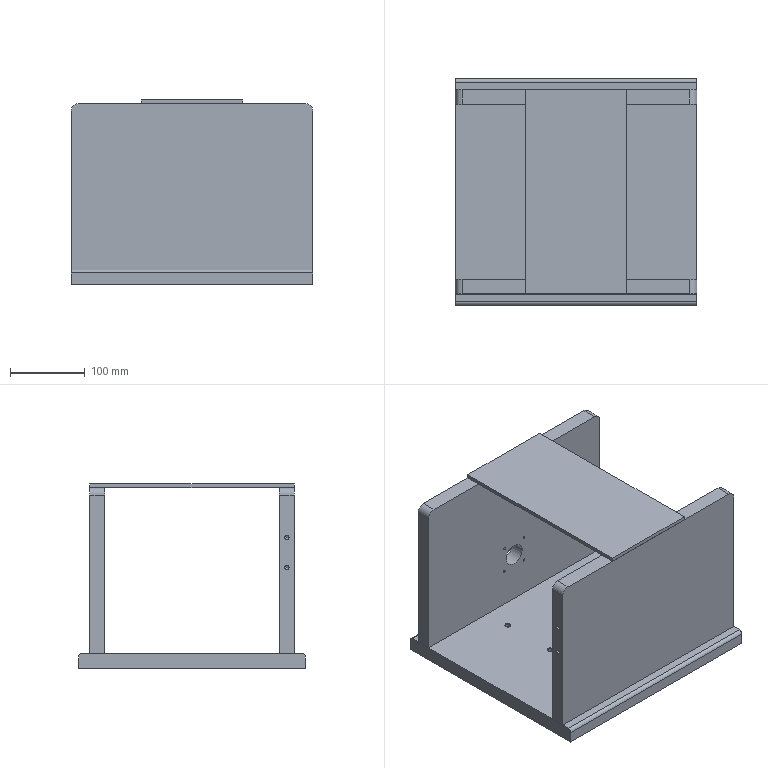Part | NX | features DATUM_CSYS 14, SKETCH 13, EXTRACT_FACE 10, HOLE PACKAGE 8, SIMPLE HOLE 8, SYMBOLIC_THREAD 8, Instance Feature 6, EXTRACT_STRING 5, EXTRUDE 5, Pattern Feature 3, BLEND 2, CHAMFER 1, Mirror Feature 1, Pattern Geometry 1 | 4 solids | 60 faces | box 324 x 304 x 247 mm | volume 5008657 mm3 | plane 24 | cylinder 19 | cone 17 | commonest cylinder face diameters 3.5 x4 5 x4 6.8 x4 20 x4 10 x2 30 x1
STEP:
#1=CARTESIAN_POINT('',(162.,289.,108.5));
#2=VERTEX_POINT('',#1);
#3=CARTESIAN_POINT('',(162.,289.,92.5));
#4=DIRECTION('',(0.,1.,0.));
#5=DIRECTION('',(0.,0.,1.));
#6=AXIS2_PLACEMENT_3D('',#3,#4,#5);
#7=CIRCLE('',#6,16.);
#8=EDGE_CURVE('',#2,#2,#7,.F.);
#9=ORIENTED_EDGE('',*,*,#8,.T.);
#10=EDGE_LOOP('',(#9));
#11=FACE_BOUND('',#10,.T.);
#12=CARTESIAN_POINT('',(143.438,289.,112.812));
#13=VERTEX_POINT('',#12);
#14=CARTESIAN_POINT('',(143.438,289.,111.062));
#15=DIRECTION('',(0.,1.,0.));
#16=DIRECTION('',(0.,0.,1.));
#17=AXIS2_PLACEMENT_3D('',#14,#15,#16);
#18=CIRCLE('',#17,1.75);
#19=EDGE_CURVE('',#13,#13,#18,.F.);
#20=ORIENTED_EDGE('',*,*,#19,.T.);
#21=EDGE_LOOP('',(#20));
#22=FACE_BOUND('',#21,.T.);
#23=CARTESIAN_POINT('',(143.438,289.,75.688));
#24=VERTEX_POINT('',#23);
#25=CARTESIAN_POINT('',(143.438,289.,73.938));
#26=DIRECTION('',(0.,1.,0.));
#27=DIRECTION('',(0.,0.,1.));
#28=AXIS2_PLACEMENT_3D('',#25,#26,#27);
#29=CIRCLE('',#28,1.75);
#30=EDGE_CURVE('',#24,#24,#29,.F.);
#31=ORIENTED_EDGE('',*,*,#30,.T.);
#32=EDGE_LOOP('',(#31));
#33=FACE_BOUND('',#32,.T.);
#34=CARTESIAN_POINT('',(180.562,289.,75.688));
#35=VERTEX_POINT('',#34);
#36=CARTESIAN_POINT('',(180.562,289.,73.938));
#37=DIRECTION('',(0.,1.,0.));
#38=DIRECTION('',(0.,0.,1.));
#39=AXIS2_PLACEMENT_3D('',#36,#37,#38);
#40=CIRCLE('',#39,1.75);
#41=EDGE_CURVE('',#35,#35,#40,.F.);
#42=ORIENTED_EDGE('',*,*,#41,.T.);
#43=EDGE_LOOP('',(#42));
#44=FACE_BOUND('',#43,.T.);
#45=CARTESIAN_POINT('',(180.562,289.,112.812));
#46=VERTEX_POINT('',#45);
#47=CARTESIAN_POINT('',(180.562,289.,111.062));
#48=DIRECTION('',(0.,1.,0.));
#49=DIRECTION('',(0.,0.,1.));
#50=AXIS2_PLACEMENT_3D('',#47,#48,#49);
#51=CIRCLE('',#50,1.75);
#52=EDGE_CURVE('',#46,#46,#51,.F.);
#53=ORIENTED_EDGE('',*,*,#52,.T.);
#54=EDGE_LOOP('',(#53));
#55=FACE_BOUND('',#54,.T.);
#56=CARTESIAN_POINT('',(0.,289.,232.));
#57=VERTEX_POINT('',#56);
#58=CARTESIAN_POINT('',(0.,289.,20.));
#59=VERTEX_POINT('',#58);
#60=CARTESIAN_POINT('',(0.,289.,242.));
#61=DIRECTION('',(0.,0.,-1.));
#62=VECTOR('',#61,1000.);
#63=LINE('',#60,#62);
#64=EDGE_CURVE('',#57,#59,#63,.T.);
#65=ORIENTED_EDGE('',*,*,#64,.F.);
#66=CARTESIAN_POINT('',(10.,289.,242.));
#67=VERTEX_POINT('',#66);
#68=CARTESIAN_POINT('',(10.,289.,232.));
#69=DIRECTION('',(0.,1.,0.));
#70=DIRECTION('',(0.,0.,1.));
#71=AXIS2_PLACEMENT_3D('',#68,#69,#70);
#72=CIRCLE('',#71,10.);
#73=EDGE_CURVE('',#57,#67,#72,.T.);
#74=ORIENTED_EDGE('',*,*,#73,.T.);
#75=CARTESIAN_POINT('',(314.,289.,242.));
#76=VERTEX_POINT('',#75);
#77=CARTESIAN_POINT('',(324.,289.,242.));
#78=DIRECTION('',(-1.,0.,0.));
#79=VECTOR('',#78,1000.);
#80=LINE('',#77,#79);
#81=EDGE_CURVE('',#76,#67,#80,.T.);
#82=ORIENTED_EDGE('',*,*,#81,.F.);
#83=CARTESIAN_POINT('',(324.,289.,232.));
#84=VERTEX_POINT('',#83);
#85=CARTESIAN_POINT('',(314.,289.,232.));
#86=DIRECTION('',(0.,1.,0.));
#87=DIRECTION('',(0.,0.,1.));
#88=AXIS2_PLACEMENT_3D('',#85,#86,#87);
#89=CIRCLE('',#88,10.);
#90=EDGE_CURVE('',#76,#84,#89,.T.);
#91=ORIENTED_EDGE('',*,*,#90,.T.);
#92=CARTESIAN_POINT('',(324.,289.,20.));
#93=VERTEX_POINT('',#92);
#94=CARTESIAN_POINT('',(324.,289.,242.));
#95=DIRECTION('',(0.,0.,-1.));
#96=VECTOR('',#95,1000.);
#97=LINE('',#94,#96);
#98=EDGE_CURVE('',#84,#93,#97,.T.);
#99=ORIENTED_EDGE('',*,*,#98,.T.);
#100=CARTESIAN_POINT('',(324.,289.,20.));
#101=DIRECTION('',(-1.,0.,0.));
#102=VECTOR('',#101,1000.);
#103=LINE('',#100,#102);
#104=EDGE_CURVE('',#93,#59,#103,.T.);
#105=ORIENTED_EDGE('',*,*,#104,.T.);
#106=EDGE_LOOP('',(#65,#74,#82,#91,#99,#105));
#107=FACE_BOUND('',#106,.T.);
#108=CARTESIAN_POINT('',(324.,289.,242.));
#109=DIRECTION('',(0.,1.,0.));
#110=DIRECTION('',(0.,0.,1.));
#111=AXIS2_PLACEMENT_3D('',#108,#109,#110);
#112=PLANE('',#111);
#113=ADVANCED_FACE('',(#11,#22,#33,#44,#55,#107),#112,.T.);
#114=CARTESIAN_POINT('',(0.,269.,20.));
#115=VERTEX_POINT('',#114);
#116=CARTESIAN_POINT('',(0.,289.,20.));
#117=DIRECTION('',(0.,-1.,0.));
#118=VECTOR('',#117,1000.);
#119=LINE('',#116,#118);
#120=EDGE_CURVE('',#59,#115,#119,.T.);
#121=ORIENTED_EDGE('',*,*,#120,.F.);
#122=ORIENTED_EDGE('',*,*,#104,.F.);
#123=CARTESIAN_POINT('',(324.,269.,20.));
#124=VERTEX_POINT('',#123);
#125=CARTESIAN_POINT('',(324.,289.,20.));
#126=DIRECTION('',(0.,-1.,0.));
#127=VECTOR('',#126,1000.);
#128=LINE('',#125,#127);
#129=EDGE_CURVE('',#93,#124,#128,.T.);
#130=ORIENTED_EDGE('',*,*,#129,.T.);
#131=CARTESIAN_POINT('',(324.,269.,20.));
#132=DIRECTION('',(-1.,0.,0.));
#133=VECTOR('',#132,1000.);
#134=LINE('',#131,#133);
#135=EDGE_CURVE('',#124,#115,#134,.T.);
#136=ORIENTED_EDGE('',*,*,#135,.T.);
#137=EDGE_LOOP('',(#121,#122,#130,#136));
#138=FACE_BOUND('',#137,.T.);
#139=CARTESIAN_POINT('',(324.,289.,20.));
#140=DIRECTION('',(0.,0.,-1.));
#141=DIRECTION('',(0.,1.,0.));
#142=AXIS2_PLACEMENT_3D('',#139,#140,#141);
#143=PLANE('',#142);
#144=ADVANCED_FACE('',(#138),#143,.T.);
#145=CARTESIAN_POINT('',(162.,269.,77.5));
#146=VERTEX_POINT('',#145);
#147=CARTESIAN_POINT('',(162.,269.,92.5));
#148=DIRECTION('',(0.,-1.,0.));
#149=DIRECTION('',(0.,0.,-1.));
#150=AXIS2_PLACEMENT_3D('',#147,#148,#149);
#151=CIRCLE('',#150,15.);
#152=EDGE_CURVE('',#146,#146,#151,.T.);
#153=ORIENTED_EDGE('',*,*,#152,.F.);
#154=EDGE_LOOP('',(#153));
#155=FACE_BOUND('',#154,.T.);
#156=CARTESIAN_POINT('',(143.438,269.,109.312));
#157=VERTEX_POINT('',#156);
#158=CARTESIAN_POINT('',(143.438,269.,111.062));
#159=DIRECTION('',(0.,-1.,0.));
#160=DIRECTION('',(0.,0.,-1.));
#161=AXIS2_PLACEMENT_3D('',#158,#159,#160);
#162=CIRCLE('',#161,1.75);
#163=EDGE_CURVE('',#157,#157,#162,.F.);
#164=ORIENTED_EDGE('',*,*,#163,.T.);
#165=EDGE_LOOP('',(#164));
#166=FACE_BOUND('',#165,.T.);
#167=CARTESIAN_POINT('',(143.438,269.,72.188));
#168=VERTEX_POINT('',#167);
#169=CARTESIAN_POINT('',(143.438,269.,73.938));
#170=DIRECTION('',(0.,-1.,0.));
#171=DIRECTION('',(0.,0.,-1.));
#172=AXIS2_PLACEMENT_3D('',#169,#170,#171);
#173=CIRCLE('',#172,1.75);
#174=EDGE_CURVE('',#168,#168,#173,.F.);
#175=ORIENTED_EDGE('',*,*,#174,.T.);
#176=EDGE_LOOP('',(#175));
#177=FACE_BOUND('',#176,.T.);
#178=CARTESIAN_POINT('',(180.562,269.,72.188));
#179=VERTEX_POINT('',#178);
#180=CARTESIAN_POINT('',(180.562,269.,73.938));
#181=DIRECTION('',(0.,-1.,0.));
#182=DIRECTION('',(0.,0.,-1.));
#183=AXIS2_PLACEMENT_3D('',#180,#181,#182);
#184=CIRCLE('',#183,1.75);
#185=EDGE_CURVE('',#179,#179,#184,.F.);
#186=ORIENTED_EDGE('',*,*,#185,.T.);
#187=EDGE_LOOP('',(#186));
#188=FACE_BOUND('',#187,.T.);
#189=CARTESIAN_POINT('',(180.562,269.,109.312));
#190=VERTEX_POINT('',#189);
#191=CARTESIAN_POINT('',(180.562,269.,111.062));
#192=DIRECTION('',(0.,-1.,0.));
#193=DIRECTION('',(0.,0.,-1.));
#194=AXIS2_PLACEMENT_3D('',#191,#192,#193);
#195=CIRCLE('',#194,1.75);
#196=EDGE_CURVE('',#190,#190,#195,.F.);
#197=ORIENTED_EDGE('',*,*,#196,.T.);
#198=EDGE_LOOP('',(#197));
#199=FACE_BOUND('',#198,.T.);
#200=CARTESIAN_POINT('',(314.,269.,242.));
#201=VERTEX_POINT('',#200);
#202=CARTESIAN_POINT('',(10.,269.,242.));
#203=VERTEX_POINT('',#202);
#204=CARTESIAN_POINT('',(324.,269.,242.));
#205=DIRECTION('',(-1.,0.,0.));
#206=VECTOR('',#205,1000.);
#207=LINE('',#204,#206);
#208=EDGE_CURVE('',#201,#203,#207,.T.);
#209=ORIENTED_EDGE('',*,*,#208,.T.);
#210=CARTESIAN_POINT('',(0.,269.,232.));
#211=VERTEX_POINT('',#210);
#212=CARTESIAN_POINT('',(10.,269.,232.));
#213=DIRECTION('',(0.,-1.,0.));
#214=DIRECTION('',(0.,0.,-1.));
#215=AXIS2_PLACEMENT_3D('',#212,#213,#214);
#216=CIRCLE('',#215,10.);
#217=EDGE_CURVE('',#203,#211,#216,.T.);
#218=ORIENTED_EDGE('',*,*,#217,.T.);
#219=CARTESIAN_POINT('',(0.,269.,20.));
#220=DIRECTION('',(0.,0.,1.));
#221=VECTOR('',#220,1000.);
#222=LINE('',#219,#221);
#223=EDGE_CURVE('',#115,#211,#222,.T.);
#224=ORIENTED_EDGE('',*,*,#223,.F.);
#225=ORIENTED_EDGE('',*,*,#135,.F.);
#226=CARTESIAN_POINT('',(324.,269.,232.));
#227=VERTEX_POINT('',#226);
#228=CARTESIAN_POINT('',(324.,269.,20.));
#229=DIRECTION('',(0.,0.,1.));
#230=VECTOR('',#229,1000.);
#231=LINE('',#228,#230);
#232=EDGE_CURVE('',#124,#227,#231,.T.);
#233=ORIENTED_EDGE('',*,*,#232,.T.);
#234=CARTESIAN_POINT('',(314.,269.,232.));
#235=DIRECTION('',(0.,-1.,0.));
#236=DIRECTION('',(0.,0.,-1.));
#237=AXIS2_PLACEMENT_3D('',#234,#235,#236);
#238=CIRCLE('',#237,10.);
#239=EDGE_CURVE('',#227,#201,#238,.T.);
#240=ORIENTED_EDGE('',*,*,#239,.T.);
#241=EDGE_LOOP('',(#209,#218,#224,#225,#233,#240));
#242=FACE_BOUND('',#241,.T.);
#243=CARTESIAN_POINT('',(324.,269.,20.));
#244=DIRECTION('',(0.,-1.,0.));
#245=DIRECTION('',(0.,0.,-1.));
#246=AXIS2_PLACEMENT_3D('',#243,#244,#245);
#247=PLANE('',#246);
#248=ADVANCED_FACE('',(#155,#166,#177,#188,#199,#242),#247,.T.);
#249=ORIENTED_EDGE('',*,*,#81,.T.);
#250=CARTESIAN_POINT('',(10.,269.,242.));
#251=DIRECTION('',(0.,1.,0.));
#252=VECTOR('',#251,1000.);
#253=LINE('',#250,#252);
#254=EDGE_CURVE('',#67,#203,#253,.F.);
#255=ORIENTED_EDGE('',*,*,#254,.T.);
#256=ORIENTED_EDGE('',*,*,#208,.F.);
#257=CARTESIAN_POINT('',(314.,289.,242.));
#258=DIRECTION('',(0.,1.,0.));
#259=VECTOR('',#258,1000.);
#260=LINE('',#257,#259);
#261=EDGE_CURVE('',#201,#76,#260,.T.);
#262=ORIENTED_EDGE('',*,*,#261,.T.);
#263=EDGE_LOOP('',(#249,#255,#256,#262));
#264=FACE_BOUND('',#263,.T.);
#265=CARTESIAN_POINT('',(324.,269.,242.));
#266=DIRECTION('',(0.,0.,1.));
#267=DIRECTION('',(1.,0.,0.));
#268=AXIS2_PLACEMENT_3D('',#265,#266,#267);
#269=PLANE('',#268);
#270=ADVANCED_FACE('',(#264),#269,.T.);
#271=ORIENTED_EDGE('',*,*,#98,.F.);
#272=CARTESIAN_POINT('',(324.,269.,232.));
#273=DIRECTION('',(0.,1.,0.));
#274=VECTOR('',#273,1000.);
#275=LINE('',#272,#274);
#276=EDGE_CURVE('',#84,#227,#275,.F.);
#277=ORIENTED_EDGE('',*,*,#276,.T.);
#278=ORIENTED_EDGE('',*,*,#232,.F.);
#279=ORIENTED_EDGE('',*,*,#129,.F.);
#280=EDGE_LOOP('',(#271,#277,#278,#279));
#281=FACE_BOUND('',#280,.T.);
#282=CARTESIAN_POINT('',(324.,0.,0.));
#283=DIRECTION('',(-1.,0.,0.));
#284=DIRECTION('',(0.,0.,1.));
#285=AXIS2_PLACEMENT_3D('',#282,#283,#284);
#286=PLANE('',#285);
#287=ADVANCED_FACE('',(#281),#286,.F.);
#288=ORIENTED_EDGE('',*,*,#223,.T.);
#289=CARTESIAN_POINT('',(0.,0.,232.));
#290=DIRECTION('',(0.,1.,0.));
#291=VECTOR('',#290,1000.);
#292=LINE('',#289,#291);
#293=EDGE_CURVE('',#211,#57,#292,.T.);
#294=ORIENTED_EDGE('',*,*,#293,.T.);
#295=ORIENTED_EDGE('',*,*,#64,.T.);
#296=ORIENTED_EDGE('',*,*,#120,.T.);
#297=EDGE_LOOP('',(#288,#294,#295,#296));
#298=FACE_BOUND('',#297,.T.);
#299=CARTESIAN_POINT('',(0.,0.,0.));
#300=DIRECTION('',(-1.,0.,0.));
#301=DIRECTION('',(0.,0.,1.));
#302=AXIS2_PLACEMENT_3D('',#299,#300,#301);
#303=PLANE('',#302);
#304=ADVANCED_FACE('',(#298),#303,.T.);
#305=ORIENTED_EDGE('',*,*,#217,.F.);
#306=ORIENTED_EDGE('',*,*,#254,.F.);
#307=ORIENTED_EDGE('',*,*,#73,.F.);
#308=ORIENTED_EDGE('',*,*,#293,.F.);
#309=EDGE_LOOP('',(#305,#306,#307,#308));
#310=FACE_BOUND('',#309,.T.);
#311=CARTESIAN_POINT('',(10.,0.,232.));
#312=DIRECTION('',(0.,1.,0.));
#313=DIRECTION('',(0.,0.,1.));
#314=AXIS2_PLACEMENT_3D('',#311,#312,#313);
#315=CYLINDRICAL_SURFACE('',#314,10.);
#316=ADVANCED_FACE('',(#310),#315,.T.);
#317=ORIENTED_EDGE('',*,*,#239,.F.);
#318=ORIENTED_EDGE('',*,*,#276,.F.);
#319=ORIENTED_EDGE('',*,*,#90,.F.);
#320=ORIENTED_EDGE('',*,*,#261,.F.);
#321=EDGE_LOOP('',(#317,#318,#319,#320));
#322=FACE_BOUND('',#321,.T.);
#323=CARTESIAN_POINT('',(314.,269.,232.));
#324=DIRECTION('',(0.,-1.,0.));
#325=DIRECTION('',(0.,0.,-1.));
#326=AXIS2_PLACEMENT_3D('',#323,#324,#325);
#327=CYLINDRICAL_SURFACE('',#326,10.);
#328=ADVANCED_FACE('',(#322),#327,.T.);
#329=ORIENTED_EDGE('',*,*,#52,.F.);
#330=EDGE_LOOP('',(#329));
#331=FACE_BOUND('',#330,.T.);
#332=ORIENTED_EDGE('',*,*,#196,.F.);
#333=EDGE_LOOP('',(#332));
#334=FACE_BOUND('',#333,.T.);
#335=CARTESIAN_POINT('',(180.562,593.,111.062));
#336=DIRECTION('',(0.,-1.,0.));
#337=DIRECTION('',(0.,0.,-1.));
#338=AXIS2_PLACEMENT_3D('',#335,#336,#337);
#339=CYLINDRICAL_SURFACE('',#338,1.75);
#340=ADVANCED_FACE('',(#331,#334),#339,.F.);
#341=ORIENTED_EDGE('',*,*,#41,.F.);
#342=EDGE_LOOP('',(#341));
#343=FACE_BOUND('',#342,.T.);
#344=ORIENTED_EDGE('',*,*,#185,.F.);
#345=EDGE_LOOP('',(#344));
#346=FACE_BOUND('',#345,.T.);
#347=CARTESIAN_POINT('',(180.562,593.,73.938));
#348=DIRECTION('',(0.,-1.,0.));
#349=DIRECTION('',(0.,0.,-1.));
#350=AXIS2_PLACEMENT_3D('',#347,#348,#349);
#351=CYLINDRICAL_SURFACE('',#350,1.75);
#352=ADVANCED_FACE('',(#343,#346),#351,.F.);
#353=ORIENTED_EDGE('',*,*,#30,.F.);
#354=EDGE_LOOP('',(#353));
#355=FACE_BOUND('',#354,.T.);
#356=ORIENTED_EDGE('',*,*,#174,.F.);
#357=EDGE_LOOP('',(#356));
#358=FACE_BOUND('',#357,.T.);
#359=CARTESIAN_POINT('',(143.438,593.,73.938));
#360=DIRECTION('',(0.,-1.,0.));
#361=DIRECTION('',(0.,0.,-1.));
#362=AXIS2_PLACEMENT_3D('',#359,#360,#361);
#363=CYLINDRICAL_SURFACE('',#362,1.75);
#364=ADVANCED_FACE('',(#355,#358),#363,.F.);
#365=ORIENTED_EDGE('',*,*,#19,.F.);
#366=EDGE_LOOP('',(#365));
#367=FACE_BOUND('',#366,.T.);
#368=ORIENTED_EDGE('',*,*,#163,.F.);
#369=EDGE_LOOP('',(#368));
#370=FACE_BOUND('',#369,.T.);
#371=CARTESIAN_POINT('',(143.438,593.,111.062));
#372=DIRECTION('',(0.,-1.,0.));
#373=DIRECTION('',(0.,0.,-1.));
#374=AXIS2_PLACEMENT_3D('',#371,#372,#373);
#375=CYLINDRICAL_SURFACE('',#374,1.75);
#376=ADVANCED_FACE('',(#367,#370),#375,.F.);
#377=CARTESIAN_POINT('',(162.,288.,107.5));
#378=VERTEX_POINT('',#377);
#379=CARTESIAN_POINT('',(162.,288.,92.5));
#380=DIRECTION('',(0.,1.,0.));
#381=DIRECTION('',(0.,0.,1.));
#382=AXIS2_PLACEMENT_3D('',#379,#380,#381);
#383=CIRCLE('',#382,15.);
#384=EDGE_CURVE('',#378,#378,#383,.T.);
#385=ORIENTED_EDGE('',*,*,#384,.T.);
#386=EDGE_LOOP('',(#385));
#387=FACE_BOUND('',#386,.T.);
#388=ORIENTED_EDGE('',*,*,#152,.T.);
#389=EDGE_LOOP('',(#388));
#390=FACE_BOUND('',#389,.T.);
#391=CARTESIAN_POINT('',(162.,593.,92.5));
#392=DIRECTION('',(0.,-1.,0.));
#393=DIRECTION('',(0.,0.,-1.));
#394=AXIS2_PLACEMENT_3D('',#391,#392,#393);
#395=CYLINDRICAL_SURFACE('',#394,15.);
#396=ADVANCED_FACE('',(#387,#390),#395,.F.);
#397=ORIENTED_EDGE('',*,*,#8,.F.);
#398=EDGE_LOOP('',(#397));
#399=FACE_BOUND('',#398,.T.);
#400=ORIENTED_EDGE('',*,*,#384,.F.);
#401=EDGE_LOOP('',(#400));
#402=FACE_BOUND('',#401,.T.);
#403=CARTESIAN_POINT('',(162.,288.,92.5));
#404=DIRECTION('',(0.,1.,0.));
#405=DIRECTION('',(0.,0.,1.));
#406=AXIS2_PLACEMENT_3D('',#403,#404,#405);
#407=CONICAL_SURFACE('',#406,15.,0.7854);
#408=ADVANCED_FACE('',(#399,#402),#407,.F.);
#409=CLOSED_SHELL('',(#113,#144,#248,#270,#287,#304,#316,#328,#340,#352,#364,#376,#396,#408));
#410=MANIFOLD_SOLID_BREP('',#409);
#411=CARTESIAN_POINT('',(94.,15.,247.));
#412=VERTEX_POINT('',#411);
#413=CARTESIAN_POINT('',(230.,15.,247.));
#414=VERTEX_POINT('',#413);
#415=CARTESIAN_POINT('',(94.,15.,247.));
#416=DIRECTION('',(1.,0.,0.));
#417=VECTOR('',#416,1000.);
#418=LINE('',#415,#417);
#419=EDGE_CURVE('',#412,#414,#418,.T.);
#420=ORIENTED_EDGE('',*,*,#419,.T.);
#421=CARTESIAN_POINT('',(230.,289.,247.));
#422=VERTEX_POINT('',#421);
#423=CARTESIAN_POINT('',(230.,289.,247.));
#424=DIRECTION('',(0.,-1.,0.));
#425=VECTOR('',#424,1000.);
#426=LINE('',#423,#425);
#427=EDGE_CURVE('',#422,#414,#426,.T.);
#428=ORIENTED_EDGE('',*,*,#427,.F.);
#429=CARTESIAN_POINT('',(94.,289.,247.));
#430=VERTEX_POINT('',#429);
#431=CARTESIAN_POINT('',(94.,289.,247.));
#432=DIRECTION('',(1.,0.,0.));
#433=VECTOR('',#432,1000.);
#434=LINE('',#431,#433);
#435=EDGE_CURVE('',#430,#422,#434,.T.);
#436=ORIENTED_EDGE('',*,*,#435,.F.);
#437=CARTESIAN_POINT('',(94.,289.,247.));
#438=DIRECTION('',(0.,-1.,0.));
#439=VECTOR('',#438,1000.);
#440=LINE('',#437,#439);
#441=EDGE_CURVE('',#430,#412,#440,.T.);
#442=ORIENTED_EDGE('',*,*,#441,.T.);
#443=EDGE_LOOP('',(#420,#428,#436,#442));
#444=FACE_BOUND('',#443,.T.);
#445=CARTESIAN_POINT('',(94.,289.,247.));
#446=DIRECTION('',(0.,0.,-1.));
#447=DIRECTION('',(-1.,0.,0.));
#448=AXIS2_PLACEMENT_3D('',#445,#446,#447);
#449=PLANE('',#448);
#450=ADVANCED_FACE('',(#444),#449,.F.);
#451=CARTESIAN_POINT('',(230.,15.,242.));
#452=VERTEX_POINT('',#451);
#453=CARTESIAN_POINT('',(230.,15.,247.));
#454=DIRECTION('',(0.,0.,-1.));
#455=VECTOR('',#454,1000.);
#456=LINE('',#453,#455);
#457=EDGE_CURVE('',#414,#452,#456,.T.);
#458=ORIENTED_EDGE('',*,*,#457,.T.);
#459=CARTESIAN_POINT('',(230.,289.,242.));
#460=VERTEX_POINT('',#459);
#461=CARTESIAN_POINT('',(230.,289.,242.));
#462=DIRECTION('',(0.,-1.,0.));
#463=VECTOR('',#462,1000.);
#464=LINE('',#461,#463);
#465=EDGE_CURVE('',#460,#452,#464,.T.);
#466=ORIENTED_EDGE('',*,*,#465,.F.);
#467=CARTESIAN_POINT('',(230.,289.,247.));
#468=DIRECTION('',(0.,0.,-1.));
#469=VECTOR('',#468,1000.);
#470=LINE('',#467,#469);
#471=EDGE_CURVE('',#422,#460,#470,.T.);
#472=ORIENTED_EDGE('',*,*,#471,.F.);
#473=ORIENTED_EDGE('',*,*,#427,.T.);
#474=EDGE_LOOP('',(#458,#466,#472,#473));
#475=FACE_BOUND('',#474,.T.);
#476=CARTESIAN_POINT('',(230.,289.,247.));
#477=DIRECTION('',(-1.,0.,0.));
#478=DIRECTION('',(0.,0.,1.));
#479=AXIS2_PLACEMENT_3D('',#476,#477,#478);
#480=PLANE('',#479);
#481=ADVANCED_FACE('',(#475),#480,.F.);
#482=CARTESIAN_POINT('',(94.,15.,242.));
#483=VERTEX_POINT('',#482);
#484=CARTESIAN_POINT('',(230.,15.,242.));
#485=DIRECTION('',(-1.,0.,0.));
#486=VECTOR('',#485,1000.);
#487=LINE('',#484,#486);
#488=EDGE_CURVE('',#452,#483,#487,.T.);
#489=ORIENTED_EDGE('',*,*,#488,.T.);
#490=CARTESIAN_POINT('',(94.,289.,242.));
#491=VERTEX_POINT('',#490);
#492=CARTESIAN_POINT('',(94.,289.,242.));
#493=DIRECTION('',(0.,-1.,0.));
#494=VECTOR('',#493,1000.);
#495=LINE('',#492,#494);
#496=EDGE_CURVE('',#491,#483,#495,.T.);
#497=ORIENTED_EDGE('',*,*,#496,.F.);
#498=CARTESIAN_POINT('',(230.,289.,242.));
#499=DIRECTION('',(-1.,0.,0.));
#500=VECTOR('',#499,1000.);
#501=LINE('',#498,#500);
#502=EDGE_CURVE('',#460,#491,#501,.T.);
#503=ORIENTED_EDGE('',*,*,#502,.F.);
#504=ORIENTED_EDGE('',*,*,#465,.T.);
#505=EDGE_LOOP('',(#489,#497,#503,#504));
#506=FACE_BOUND('',#505,.T.);
#507=CARTESIAN_POINT('',(230.,289.,242.));
#508=DIRECTION('',(0.,0.,1.));
#509=DIRECTION('',(1.,0.,0.));
#510=AXIS2_PLACEMENT_3D('',#507,#508,#509);
#511=PLANE('',#510);
#512=ADVANCED_FACE('',(#506),#511,.F.);
#513=CARTESIAN_POINT('',(94.,15.,242.));
#514=DIRECTION('',(0.,0.,1.));
#515=VECTOR('',#514,1000.);
#516=LINE('',#513,#515);
#517=EDGE_CURVE('',#483,#412,#516,.T.);
#518=ORIENTED_EDGE('',*,*,#517,.T.);
#519=ORIENTED_EDGE('',*,*,#441,.F.);
#520=CARTESIAN_POINT('',(94.,289.,242.));
#521=DIRECTION('',(0.,0.,1.));
#522=VECTOR('',#521,1000.);
#523=LINE('',#520,#522);
#524=EDGE_CURVE('',#491,#430,#523,.T.);
#525=ORIENTED_EDGE('',*,*,#524,.F.);
#526=ORIENTED_EDGE('',*,*,#496,.T.);
#527=EDGE_LOOP('',(#518,#519,#525,#526));
#528=FACE_BOUND('',#527,.T.);
#529=CARTESIAN_POINT('',(94.,289.,242.));
#530=DIRECTION('',(1.,0.,0.));
#531=DIRECTION('',(0.,0.,-1.));
#532=AXIS2_PLACEMENT_3D('',#529,#530,#531);
#533=PLANE('',#532);
#534=ADVANCED_FACE('',(#528),#533,.F.);
#535=ORIENTED_EDGE('',*,*,#435,.T.);
#536=ORIENTED_EDGE('',*,*,#471,.T.);
#537=ORIENTED_EDGE('',*,*,#502,.T.);
#538=ORIENTED_EDGE('',*,*,#524,.T.);
#539=EDGE_LOOP('',(#535,#536,#537,#538));
#540=FACE_BOUND('',#539,.T.);
#541=CARTESIAN_POINT('',(0.,289.,0.));
#542=DIRECTION('',(0.,1.,0.));
#543=DIRECTION('',(0.,0.,1.));
#544=AXIS2_PLACEMENT_3D('',#541,#542,#543);
#545=PLANE('',#544);
#546=ADVANCED_FACE('',(#540),#545,.T.);
#547=ORIENTED_EDGE('',*,*,#419,.F.);
#548=ORIENTED_EDGE('',*,*,#517,.F.);
#549=ORIENTED_EDGE('',*,*,#488,.F.);
#550=ORIENTED_EDGE('',*,*,#457,.F.);
#551=EDGE_LOOP('',(#547,#548,#549,#550));
#552=FACE_BOUND('',#551,.T.);
#553=CARTESIAN_POINT('',(0.,15.,0.));
#554=DIRECTION('',(0.,1.,0.));
#555=DIRECTION('',(0.,0.,1.));
#556=AXIS2_PLACEMENT_3D('',#553,#554,#555);
#557=PLANE('',#556);
#558=ADVANCED_FACE('',(#552),#557,.F.);
#559=CLOSED_SHELL('',(#450,#481,#512,#534,#546,#558));
#560=MANIFOLD_SOLID_BREP('',#559);
#561=CARTESIAN_POINT('',(212.,147.,20.));
#562=VERTEX_POINT('',#561);
#563=CARTESIAN_POINT('',(212.,151.,20.));
#564=DIRECTION('',(0.,0.,1.));
#565=DIRECTION('',(0.,-1.,0.));
#566=AXIS2_PLACEMENT_3D('',#563,#564,#565);
#567=CIRCLE('',#566,4.);
#568=EDGE_CURVE('',#562,#562,#567,.F.);
#569=ORIENTED_EDGE('',*,*,#568,.T.);
#570=EDGE_LOOP('',(#569));
#571=FACE_BOUND('',#570,.T.);
#572=CARTESIAN_POINT('',(212.,227.,20.));
#573=VERTEX_POINT('',#572);
#574=CARTESIAN_POINT('',(212.,231.,20.));
#575=DIRECTION('',(0.,0.,1.));
#576=DIRECTION('',(0.,-1.,0.));
#577=AXIS2_PLACEMENT_3D('',#574,#575,#576);
#578=CIRCLE('',#577,4.);
#579=EDGE_CURVE('',#573,#573,#578,.F.);
#580=ORIENTED_EDGE('',*,*,#579,.T.);
#581=EDGE_LOOP('',(#580));
#582=FACE_BOUND('',#581,.T.);
#583=CARTESIAN_POINT('',(112.,147.,20.));
#584=VERTEX_POINT('',#583);
#585=CARTESIAN_POINT('',(112.,151.,20.));
#586=DIRECTION('',(0.,0.,1.));
#587=DIRECTION('',(0.,-1.,0.));
#588=AXIS2_PLACEMENT_3D('',#585,#586,#587);
#589=CIRCLE('',#588,4.);
#590=EDGE_CURVE('',#584,#584,#589,.F.);
#591=ORIENTED_EDGE('',*,*,#590,.T.);
#592=EDGE_LOOP('',(#591));
#593=FACE_BOUND('',#592,.T.);
#594=CARTESIAN_POINT('',(112.,227.,20.));
#595=VERTEX_POINT('',#594);
#596=CARTESIAN_POINT('',(112.,231.,20.));
#597=DIRECTION('',(0.,0.,1.));
#598=DIRECTION('',(0.,-1.,0.));
#599=AXIS2_PLACEMENT_3D('',#596,#597,#598);
#600=CIRCLE('',#599,4.);
#601=EDGE_CURVE('',#595,#595,#600,.F.);
#602=ORIENTED_EDGE('',*,*,#601,.T.);
#603=EDGE_LOOP('',(#602));
#604=FACE_BOUND('',#603,.T.);
#605=CARTESIAN_POINT('',(324.,5.,20.));
#606=VERTEX_POINT('',#605);
#607=CARTESIAN_POINT('',(324.,299.,20.));
#608=VERTEX_POINT('',#607);
#609=CARTESIAN_POINT('',(324.,0.,20.));
#610=DIRECTION('',(0.,1.,0.));
#611=VECTOR('',#610,1000.);
#612=LINE('',#609,#611);
#613=EDGE_CURVE('',#606,#608,#612,.T.);
#614=ORIENTED_EDGE('',*,*,#613,.T.);
#615=CARTESIAN_POINT('',(0.,299.,20.));
#616=VERTEX_POINT('',#615);
#617=CARTESIAN_POINT('',(324.,299.,20.));
#618=DIRECTION('',(-1.,0.,0.));
#619=VECTOR('',#618,1000.);
#620=LINE('',#617,#619);
#621=EDGE_CURVE('',#608,#616,#620,.T.);
#622=ORIENTED_EDGE('',*,*,#621,.T.);
#623=CARTESIAN_POINT('',(0.,5.,20.));
#624=VERTEX_POINT('',#623);
#625=CARTESIAN_POINT('',(0.,0.,20.));
#626=DIRECTION('',(0.,1.,0.));
#627=VECTOR('',#626,1000.);
#628=LINE('',#625,#627);
#629=EDGE_CURVE('',#624,#616,#628,.T.);
#630=ORIENTED_EDGE('',*,*,#629,.F.);
#631=CARTESIAN_POINT('',(324.,5.,20.));
#632=DIRECTION('',(-1.,0.,0.));
#633=VECTOR('',#632,1000.);
#634=LINE('',#631,#633);
#635=EDGE_CURVE('',#624,#606,#634,.F.);
#636=ORIENTED_EDGE('',*,*,#635,.T.);
#637=EDGE_LOOP('',(#614,#622,#630,#636));
#638=FACE_BOUND('',#637,.T.);
#639=CARTESIAN_POINT('',(324.,0.,20.));
#640=DIRECTION('',(0.,0.,1.));
#641=DIRECTION('',(0.,-1.,0.));
#642=AXIS2_PLACEMENT_3D('',#639,#640,#641);
#643=PLANE('',#642);
#644=ADVANCED_FACE('',(#571,#582,#593,#604,#638),#643,.T.);
#645=CARTESIAN_POINT('',(0.,304.,15.));
#646=VERTEX_POINT('',#645);
#647=CARTESIAN_POINT('',(0.,304.,0.));
#648=VERTEX_POINT('',#647);
#649=CARTESIAN_POINT('',(0.,304.,20.));
#650=DIRECTION('',(0.,0.,-1.));
#651=VECTOR('',#650,1000.);
#652=LINE('',#649,#651);
#653=EDGE_CURVE('',#646,#648,#652,.T.);
#654=ORIENTED_EDGE('',*,*,#653,.F.);
#655=CARTESIAN_POINT('',(324.,304.,15.));
#656=VERTEX_POINT('',#655);
#657=CARTESIAN_POINT('',(324.,304.,15.));
#658=DIRECTION('',(-1.,0.,0.));
#659=VECTOR('',#658,1000.);
#660=LINE('',#657,#659);
#661=EDGE_CURVE('',#646,#656,#660,.F.);
#662=ORIENTED_EDGE('',*,*,#661,.T.);
#663=CARTESIAN_POINT('',(324.,304.,0.));
#664=VERTEX_POINT('',#663);
#665=CARTESIAN_POINT('',(324.,304.,20.));
#666=DIRECTION('',(0.,0.,-1.));
#667=VECTOR('',#666,1000.);
#668=LINE('',#665,#667);
#669=EDGE_CURVE('',#656,#664,#668,.T.);
#670=ORIENTED_EDGE('',*,*,#669,.T.);
#671=CARTESIAN_POINT('',(324.,304.,0.));
#672=DIRECTION('',(-1.,0.,0.));
#673=VECTOR('',#672,1000.);
#674=LINE('',#671,#673);
#675=EDGE_CURVE('',#664,#648,#674,.T.);
#676=ORIENTED_EDGE('',*,*,#675,.T.);
#677=EDGE_LOOP('',(#654,#662,#670,#676));
#678=FACE_BOUND('',#677,.T.);
#679=CARTESIAN_POINT('',(324.,304.,20.));
#680=DIRECTION('',(0.,1.,0.));
#681=DIRECTION('',(0.,0.,1.));
#682=AXIS2_PLACEMENT_3D('',#679,#680,#681);
#683=PLANE('',#682);
#684=ADVANCED_FACE('',(#678),#683,.T.);
#685=CARTESIAN_POINT('',(212.,155.,0.));
#686=VERTEX_POINT('',#685);
#687=CARTESIAN_POINT('',(212.,151.,0.));
#688=DIRECTION('',(0.,0.,-1.));
#689=DIRECTION('',(0.,1.,0.));
#690=AXIS2_PLACEMENT_3D('',#687,#688,#689);
#691=CIRCLE('',#690,4.);
#692=EDGE_CURVE('',#686,#686,#691,.F.);
#693=ORIENTED_EDGE('',*,*,#692,.T.);
#694=EDGE_LOOP('',(#693));
#695=FACE_BOUND('',#694,.T.);
#696=CARTESIAN_POINT('',(212.,235.,0.));
#697=VERTEX_POINT('',#696);
#698=CARTESIAN_POINT('',(212.,231.,0.));
#699=DIRECTION('',(0.,0.,-1.));
#700=DIRECTION('',(0.,1.,0.));
#701=AXIS2_PLACEMENT_3D('',#698,#699,#700);
#702=CIRCLE('',#701,4.);
#703=EDGE_CURVE('',#697,#697,#702,.F.);
#704=ORIENTED_EDGE('',*,*,#703,.T.);
#705=EDGE_LOOP('',(#704));
#706=FACE_BOUND('',#705,.T.);
#707=CARTESIAN_POINT('',(112.,155.,0.));
#708=VERTEX_POINT('',#707);
#709=CARTESIAN_POINT('',(112.,151.,0.));
#710=DIRECTION('',(0.,0.,-1.));
#711=DIRECTION('',(0.,1.,0.));
#712=AXIS2_PLACEMENT_3D('',#709,#710,#711);
#713=CIRCLE('',#712,4.);
#714=EDGE_CURVE('',#708,#708,#713,.F.);
#715=ORIENTED_EDGE('',*,*,#714,.T.);
#716=EDGE_LOOP('',(#715));
#717=FACE_BOUND('',#716,.T.);
#718=CARTESIAN_POINT('',(112.,235.,0.));
#719=VERTEX_POINT('',#718);
#720=CARTESIAN_POINT('',(112.,231.,0.));
#721=DIRECTION('',(0.,0.,-1.));
#722=DIRECTION('',(0.,1.,0.));
#723=AXIS2_PLACEMENT_3D('',#720,#721,#722);
#724=CIRCLE('',#723,4.);
#725=EDGE_CURVE('',#719,#719,#724,.F.);
#726=ORIENTED_EDGE('',*,*,#725,.T.);
#727=EDGE_LOOP('',(#726));
#728=FACE_BOUND('',#727,.T.);
#729=CARTESIAN_POINT('',(0.,0.,0.));
#730=VERTEX_POINT('',#729);
#731=CARTESIAN_POINT('',(0.,304.,0.));
#732=DIRECTION('',(0.,-1.,0.));
#733=VECTOR('',#732,1000.);
#734=LINE('',#731,#733);
#735=EDGE_CURVE('',#648,#730,#734,.T.);
#736=ORIENTED_EDGE('',*,*,#735,.F.);
#737=ORIENTED_EDGE('',*,*,#675,.F.);
#738=CARTESIAN_POINT('',(324.,0.,0.));
#739=VERTEX_POINT('',#738);
#740=CARTESIAN_POINT('',(324.,304.,0.));
#741=DIRECTION('',(0.,-1.,0.));
#742=VECTOR('',#741,1000.);
#743=LINE('',#740,#742);
#744=EDGE_CURVE('',#664,#739,#743,.T.);
#745=ORIENTED_EDGE('',*,*,#744,.T.);
#746=CARTESIAN_POINT('',(324.,0.,0.));
#747=DIRECTION('',(-1.,0.,0.));
#748=VECTOR('',#747,1000.);
#749=LINE('',#746,#748);
#750=EDGE_CURVE('',#739,#730,#749,.T.);
#751=ORIENTED_EDGE('',*,*,#750,.T.);
#752=EDGE_LOOP('',(#736,#737,#745,#751));
#753=FACE_BOUND('',#752,.T.);
#754=CARTESIAN_POINT('',(324.,304.,0.));
#755=DIRECTION('',(0.,0.,-1.));
#756=DIRECTION('',(0.,1.,0.));
#757=AXIS2_PLACEMENT_3D('',#754,#755,#756);
#758=PLANE('',#757);
#759=ADVANCED_FACE('',(#695,#706,#717,#728,#753),#758,.T.);
#760=CARTESIAN_POINT('',(324.,0.,15.));
#761=VERTEX_POINT('',#760);
#762=CARTESIAN_POINT('',(324.,0.,0.));
#763=DIRECTION('',(0.,0.,1.));
#764=VECTOR('',#763,1000.);
#765=LINE('',#762,#764);
#766=EDGE_CURVE('',#739,#761,#765,.T.);
#767=ORIENTED_EDGE('',*,*,#766,.T.);
#768=CARTESIAN_POINT('',(0.,0.,15.));
#769=VERTEX_POINT('',#768);
#770=CARTESIAN_POINT('',(324.,0.,15.));
#771=DIRECTION('',(-1.,0.,0.));
#772=VECTOR('',#771,1000.);
#773=LINE('',#770,#772);
#774=EDGE_CURVE('',#761,#769,#773,.T.);
#775=ORIENTED_EDGE('',*,*,#774,.T.);
#776=CARTESIAN_POINT('',(0.,0.,0.));
#777=DIRECTION('',(0.,0.,1.));
#778=VECTOR('',#777,1000.);
#779=LINE('',#776,#778);
#780=EDGE_CURVE('',#730,#769,#779,.T.);
#781=ORIENTED_EDGE('',*,*,#780,.F.);
#782=ORIENTED_EDGE('',*,*,#750,.F.);
#783=EDGE_LOOP('',(#767,#775,#781,#782));
#784=FACE_BOUND('',#783,.T.);
#785=CARTESIAN_POINT('',(324.,0.,0.));
#786=DIRECTION('',(0.,-1.,0.));
#787=DIRECTION('',(0.,0.,-1.));
#788=AXIS2_PLACEMENT_3D('',#785,#786,#787);
#789=PLANE('',#788);
#790=ADVANCED_FACE('',(#784),#789,.T.);
#791=ORIENTED_EDGE('',*,*,#669,.F.);
#792=CARTESIAN_POINT('',(324.,299.,15.));
#793=DIRECTION('',(-1.,0.,0.));
#794=DIRECTION('',(0.,0.,1.));
#795=AXIS2_PLACEMENT_3D('',#792,#793,#794);
#796=CIRCLE('',#795,5.);
#797=EDGE_CURVE('',#656,#608,#796,.F.);
#798=ORIENTED_EDGE('',*,*,#797,.T.);
#799=ORIENTED_EDGE('',*,*,#613,.F.);
#800=CARTESIAN_POINT('',(324.,5.,15.));
#801=DIRECTION('',(-1.,0.,0.));
#802=DIRECTION('',(0.,0.,1.));
#803=AXIS2_PLACEMENT_3D('',#800,#801,#802);
#804=CIRCLE('',#803,5.);
#805=EDGE_CURVE('',#606,#761,#804,.F.);
#806=ORIENTED_EDGE('',*,*,#805,.T.);
#807=ORIENTED_EDGE('',*,*,#766,.F.);
#808=ORIENTED_EDGE('',*,*,#744,.F.);
#809=EDGE_LOOP('',(#791,#798,#799,#806,#807,#808));
#810=FACE_BOUND('',#809,.T.);
#811=CARTESIAN_POINT('',(324.,0.,0.));
#812=DIRECTION('',(-1.,0.,0.));
#813=DIRECTION('',(0.,0.,1.));
#814=AXIS2_PLACEMENT_3D('',#811,#812,#813);
#815=PLANE('',#814);
#816=ADVANCED_FACE('',(#810),#815,.F.);
#817=ORIENTED_EDGE('',*,*,#629,.T.);
#818=CARTESIAN_POINT('',(0.,299.,15.));
#819=DIRECTION('',(-1.,0.,0.));
#820=DIRECTION('',(0.,0.,1.));
#821=AXIS2_PLACEMENT_3D('',#818,#819,#820);
#822=CIRCLE('',#821,5.);
#823=EDGE_CURVE('',#616,#646,#822,.T.);
#824=ORIENTED_EDGE('',*,*,#823,.T.);
#825=ORIENTED_EDGE('',*,*,#653,.T.);
#826=ORIENTED_EDGE('',*,*,#735,.T.);
#827=ORIENTED_EDGE('',*,*,#780,.T.);
#828=CARTESIAN_POINT('',(0.,5.,15.));
#829=DIRECTION('',(-1.,0.,0.));
#830=DIRECTION('',(0.,0.,1.));
#831=AXIS2_PLACEMENT_3D('',#828,#829,#830);
#832=CIRCLE('',#831,5.);
#833=EDGE_CURVE('',#769,#624,#832,.T.);
#834=ORIENTED_EDGE('',*,*,#833,.T.);
#835=EDGE_LOOP('',(#817,#824,#825,#826,#827,#834));
#836=FACE_BOUND('',#835,.T.);
#837=CARTESIAN_POINT('',(0.,0.,0.));
#838=DIRECTION('',(-1.,0.,0.));
#839=DIRECTION('',(0.,0.,1.));
#840=AXIS2_PLACEMENT_3D('',#837,#838,#839);
#841=PLANE('',#840);
#842=ADVANCED_FACE('',(#836),#841,.T.);
#843=ORIENTED_EDGE('',*,*,#797,.F.);
#844=ORIENTED_EDGE('',*,*,#661,.F.);
#845=ORIENTED_EDGE('',*,*,#823,.F.);
#846=ORIENTED_EDGE('',*,*,#621,.F.);
#847=EDGE_LOOP('',(#843,#844,#845,#846));
#848=FACE_BOUND('',#847,.T.);
#849=CARTESIAN_POINT('',(324.,299.,15.));
#850=DIRECTION('',(-1.,0.,0.));
#851=DIRECTION('',(0.,0.,1.));
#852=AXIS2_PLACEMENT_3D('',#849,#850,#851);
#853=CYLINDRICAL_SURFACE('',#852,5.);
#854=ADVANCED_FACE('',(#848),#853,.T.);
#855=ORIENTED_EDGE('',*,*,#805,.F.);
#856=ORIENTED_EDGE('',*,*,#635,.F.);
#857=ORIENTED_EDGE('',*,*,#833,.F.);
#858=ORIENTED_EDGE('',*,*,#774,.F.);
#859=EDGE_LOOP('',(#855,#856,#857,#858));
#860=FACE_BOUND('',#859,.T.);
#861=CARTESIAN_POINT('',(324.,5.,15.));
#862=DIRECTION('',(-1.,0.,0.));
#863=DIRECTION('',(0.,0.,1.));
#864=AXIS2_PLACEMENT_3D('',#861,#862,#863);
#865=CYLINDRICAL_SURFACE('',#864,5.);
#866=ADVANCED_FACE('',(#860),#865,.T.);
#867=CARTESIAN_POINT('',(108.6,231.,0.6));
#868=VERTEX_POINT('',#867);
#869=CARTESIAN_POINT('',(112.,231.,0.6));
#870=DIRECTION('',(0.,0.,-1.));
#871=DIRECTION('',(-1.,0.,0.));
#872=AXIS2_PLACEMENT_3D('',#869,#870,#871);
#873=CIRCLE('',#872,3.4);
#874=EDGE_CURVE('',#868,#868,#873,.T.);
#875=ORIENTED_EDGE('',*,*,#874,.T.);
#876=EDGE_LOOP('',(#875));
#877=FACE_BOUND('',#876,.T.);
#878=CARTESIAN_POINT('',(115.4,231.,19.4));
#879=VERTEX_POINT('',#878);
#880=CARTESIAN_POINT('',(112.,231.,19.4));
#881=DIRECTION('',(0.,0.,1.));
#882=DIRECTION('',(1.,0.,0.));
#883=AXIS2_PLACEMENT_3D('',#880,#881,#882);
#884=CIRCLE('',#883,3.4);
#885=EDGE_CURVE('',#879,#879,#884,.T.);
#886=ORIENTED_EDGE('',*,*,#885,.T.);
#887=EDGE_LOOP('',(#886));
#888=FACE_BOUND('',#887,.T.);
#889=CARTESIAN_POINT('',(112.,231.,20.));
#890=DIRECTION('',(0.,0.,-1.));
#891=DIRECTION('',(0.,1.,0.));
#892=AXIS2_PLACEMENT_3D('',#889,#890,#891);
#893=CYLINDRICAL_SURFACE('',#892,3.4);
#894=ADVANCED_FACE('',(#877,#888),#893,.F.);
#895=ORIENTED_EDGE('',*,*,#885,.F.);
#896=EDGE_LOOP('',(#895));
#897=FACE_BOUND('',#896,.T.);
#898=ORIENTED_EDGE('',*,*,#601,.F.);
#899=EDGE_LOOP('',(#898));
#900=FACE_BOUND('',#899,.T.);
#901=CARTESIAN_POINT('',(112.,231.,20.));
#902=DIRECTION('',(0.,0.,1.));
#903=DIRECTION('',(1.,0.,0.));
#904=AXIS2_PLACEMENT_3D('',#901,#902,#903);
#905=CONICAL_SURFACE('',#904,4.,0.7854);
#906=ADVANCED_FACE('',(#897,#900),#905,.F.);
#907=ORIENTED_EDGE('',*,*,#725,.F.);
#908=EDGE_LOOP('',(#907));
#909=FACE_BOUND('',#908,.T.);
#910=ORIENTED_EDGE('',*,*,#874,.F.);
#911=EDGE_LOOP('',(#910));
#912=FACE_BOUND('',#911,.T.);
#913=CARTESIAN_POINT('',(112.,231.,0.6));
#914=DIRECTION('',(0.,0.,-1.));
#915=DIRECTION('',(-1.,0.,0.));
#916=AXIS2_PLACEMENT_3D('',#913,#914,#915);
#917=CONICAL_SURFACE('',#916,3.4,0.7854);
#918=ADVANCED_FACE('',(#909,#912),#917,.F.);
#919=CARTESIAN_POINT('',(108.6,151.,0.6));
#920=VERTEX_POINT('',#919);
#921=CARTESIAN_POINT('',(112.,151.,0.6));
#922=DIRECTION('',(0.,0.,-1.));
#923=DIRECTION('',(-1.,0.,0.));
#924=AXIS2_PLACEMENT_3D('',#921,#922,#923);
#925=CIRCLE('',#924,3.4);
#926=EDGE_CURVE('',#920,#920,#925,.T.);
#927=ORIENTED_EDGE('',*,*,#926,.T.);
#928=EDGE_LOOP('',(#927));
#929=FACE_BOUND('',#928,.T.);
#930=CARTESIAN_POINT('',(115.4,151.,19.4));
#931=VERTEX_POINT('',#930);
#932=CARTESIAN_POINT('',(112.,151.,19.4));
#933=DIRECTION('',(0.,0.,1.));
#934=DIRECTION('',(1.,0.,0.));
#935=AXIS2_PLACEMENT_3D('',#932,#933,#934);
#936=CIRCLE('',#935,3.4);
#937=EDGE_CURVE('',#931,#931,#936,.T.);
#938=ORIENTED_EDGE('',*,*,#937,.T.);
#939=EDGE_LOOP('',(#938));
#940=FACE_BOUND('',#939,.T.);
#941=CARTESIAN_POINT('',(112.,151.,20.));
#942=DIRECTION('',(0.,0.,-1.));
#943=DIRECTION('',(0.,1.,0.));
#944=AXIS2_PLACEMENT_3D('',#941,#942,#943);
#945=CYLINDRICAL_SURFACE('',#944,3.4);
#946=ADVANCED_FACE('',(#929,#940),#945,.F.);
#947=ORIENTED_EDGE('',*,*,#937,.F.);
#948=EDGE_LOOP('',(#947));
#949=FACE_BOUND('',#948,.T.);
#950=ORIENTED_EDGE('',*,*,#590,.F.);
#951=EDGE_LOOP('',(#950));
#952=FACE_BOUND('',#951,.T.);
#953=CARTESIAN_POINT('',(112.,151.,20.));
#954=DIRECTION('',(0.,0.,1.));
#955=DIRECTION('',(1.,0.,0.));
#956=AXIS2_PLACEMENT_3D('',#953,#954,#955);
#957=CONICAL_SURFACE('',#956,4.,0.7854);
#958=ADVANCED_FACE('',(#949,#952),#957,.F.);
#959=ORIENTED_EDGE('',*,*,#714,.F.);
#960=EDGE_LOOP('',(#959));
#961=FACE_BOUND('',#960,.T.);
#962=ORIENTED_EDGE('',*,*,#926,.F.);
#963=EDGE_LOOP('',(#962));
#964=FACE_BOUND('',#963,.T.);
#965=CARTESIAN_POINT('',(112.,151.,0.6));
#966=DIRECTION('',(0.,0.,-1.));
#967=DIRECTION('',(-1.,0.,0.));
#968=AXIS2_PLACEMENT_3D('',#965,#966,#967);
#969=CONICAL_SURFACE('',#968,3.4,0.7854);
#970=ADVANCED_FACE('',(#961,#964),#969,.F.);
#971=CARTESIAN_POINT('',(208.6,231.,0.6));
#972=VERTEX_POINT('',#971);
#973=CARTESIAN_POINT('',(212.,231.,0.6));
#974=DIRECTION('',(0.,0.,-1.));
#975=DIRECTION('',(-1.,0.,0.));
#976=AXIS2_PLACEMENT_3D('',#973,#974,#975);
#977=CIRCLE('',#976,3.4);
#978=EDGE_CURVE('',#972,#972,#977,.T.);
#979=ORIENTED_EDGE('',*,*,#978,.T.);
#980=EDGE_LOOP('',(#979));
#981=FACE_BOUND('',#980,.T.);
#982=CARTESIAN_POINT('',(215.4,231.,19.4));
#983=VERTEX_POINT('',#982);
#984=CARTESIAN_POINT('',(212.,231.,19.4));
#985=DIRECTION('',(0.,0.,1.));
#986=DIRECTION('',(1.,0.,0.));
#987=AXIS2_PLACEMENT_3D('',#984,#985,#986);
#988=CIRCLE('',#987,3.4);
#989=EDGE_CURVE('',#983,#983,#988,.T.);
#990=ORIENTED_EDGE('',*,*,#989,.T.);
#991=EDGE_LOOP('',(#990));
#992=FACE_BOUND('',#991,.T.);
#993=CARTESIAN_POINT('',(212.,231.,20.));
#994=DIRECTION('',(0.,0.,-1.));
#995=DIRECTION('',(0.,1.,0.));
#996=AXIS2_PLACEMENT_3D('',#993,#994,#995);
#997=CYLINDRICAL_SURFACE('',#996,3.4);
#998=ADVANCED_FACE('',(#981,#992),#997,.F.);
#999=ORIENTED_EDGE('',*,*,#989,.F.);
#1000=EDGE_LOOP('',(#999));
#1001=FACE_BOUND('',#1000,.T.);
#1002=ORIENTED_EDGE('',*,*,#579,.F.);
#1003=EDGE_LOOP('',(#1002));
#1004=FACE_BOUND('',#1003,.T.);
#1005=CARTESIAN_POINT('',(212.,231.,20.));
#1006=DIRECTION('',(0.,0.,1.));
#1007=DIRECTION('',(1.,0.,0.));
#1008=AXIS2_PLACEMENT_3D('',#1005,#1006,#1007);
#1009=CONICAL_SURFACE('',#1008,4.,0.7854);
#1010=ADVANCED_FACE('',(#1001,#1004),#1009,.F.);
#1011=ORIENTED_EDGE('',*,*,#703,.F.);
#1012=EDGE_LOOP('',(#1011));
#1013=FACE_BOUND('',#1012,.T.);
#1014=ORIENTED_EDGE('',*,*,#978,.F.);
#1015=EDGE_LOOP('',(#1014));
#1016=FACE_BOUND('',#1015,.T.);
#1017=CARTESIAN_POINT('',(212.,231.,0.6));
#1018=DIRECTION('',(0.,0.,-1.));
#1019=DIRECTION('',(-1.,0.,0.));
#1020=AXIS2_PLACEMENT_3D('',#1017,#1018,#1019);
#1021=CONICAL_SURFACE('',#1020,3.4,0.7854);
#1022=ADVANCED_FACE('',(#1013,#1016),#1021,.F.);
#1023=CARTESIAN_POINT('',(208.6,151.,0.6));
#1024=VERTEX_POINT('',#1023);
#1025=CARTESIAN_POINT('',(212.,151.,0.6));
#1026=DIRECTION('',(0.,0.,-1.));
#1027=DIRECTION('',(-1.,0.,0.));
#1028=AXIS2_PLACEMENT_3D('',#1025,#1026,#1027);
#1029=CIRCLE('',#1028,3.4);
#1030=EDGE_CURVE('',#1024,#1024,#1029,.T.);
#1031=ORIENTED_EDGE('',*,*,#1030,.T.);
#1032=EDGE_LOOP('',(#1031));
#1033=FACE_BOUND('',#1032,.T.);
#1034=CARTESIAN_POINT('',(215.4,151.,19.4));
#1035=VERTEX_POINT('',#1034);
#1036=CARTESIAN_POINT('',(212.,151.,19.4));
#1037=DIRECTION('',(0.,0.,1.));
#1038=DIRECTION('',(1.,0.,0.));
#1039=AXIS2_PLACEMENT_3D('',#1036,#1037,#1038);
#1040=CIRCLE('',#1039,3.4);
#1041=EDGE_CURVE('',#1035,#1035,#1040,.T.);
#1042=ORIENTED_EDGE('',*,*,#1041,.T.);
#1043=EDGE_LOOP('',(#1042));
#1044=FACE_BOUND('',#1043,.T.);
#1045=CARTESIAN_POINT('',(212.,151.,20.));
#1046=DIRECTION('',(0.,0.,-1.));
#1047=DIRECTION('',(0.,1.,0.));
#1048=AXIS2_PLACEMENT_3D('',#1045,#1046,#1047);
#1049=CYLINDRICAL_SURFACE('',#1048,3.4);
#1050=ADVANCED_FACE('',(#1033,#1044),#1049,.F.);
#1051=ORIENTED_EDGE('',*,*,#1041,.F.);
#1052=EDGE_LOOP('',(#1051));
#1053=FACE_BOUND('',#1052,.T.);
#1054=ORIENTED_EDGE('',*,*,#568,.F.);
#1055=EDGE_LOOP('',(#1054));
#1056=FACE_BOUND('',#1055,.T.);
#1057=CARTESIAN_POINT('',(212.,151.,20.));
#1058=DIRECTION('',(0.,0.,1.));
#1059=DIRECTION('',(1.,0.,0.));
#1060=AXIS2_PLACEMENT_3D('',#1057,#1058,#1059);
#1061=CONICAL_SURFACE('',#1060,4.,0.7854);
#1062=ADVANCED_FACE('',(#1053,#1056),#1061,.F.);
#1063=ORIENTED_EDGE('',*,*,#692,.F.);
#1064=EDGE_LOOP('',(#1063));
#1065=FACE_BOUND('',#1064,.T.);
#1066=ORIENTED_EDGE('',*,*,#1030,.F.);
#1067=EDGE_LOOP('',(#1066));
#1068=FACE_BOUND('',#1067,.T.);
#1069=CARTESIAN_POINT('',(212.,151.,0.6));
#1070=DIRECTION('',(0.,0.,-1.));
#1071=DIRECTION('',(-1.,0.,0.));
#1072=AXIS2_PLACEMENT_3D('',#1069,#1070,#1071);
#1073=CONICAL_SURFACE('',#1072,3.4,0.7854);
#1074=ADVANCED_FACE('',(#1065,#1068),#1073,.F.);
#1075=CLOSED_SHELL('',(#644,#684,#759,#790,#816,#842,#854,#866,#894,#906,#918,#946,#958,#970,#998,#1010,#1022,#1050,#1062,#1074));
#1076=MANIFOLD_SOLID_BREP('',#1075);
#1077=CARTESIAN_POINT('',(0.,35.,232.));
#1078=VERTEX_POINT('',#1077);
#1079=CARTESIAN_POINT('',(0.,35.,20.));
#1080=VERTEX_POINT('',#1079);
#1081=CARTESIAN_POINT('',(0.,35.,242.));
#1082=DIRECTION('',(0.,0.,-1.));
#1083=VECTOR('',#1082,1000.);
#1084=LINE('',#1081,#1083);
#1085=EDGE_CURVE('',#1078,#1080,#1084,.T.);
#1086=ORIENTED_EDGE('',*,*,#1085,.F.);
#1087=CARTESIAN_POINT('',(10.,35.,242.));
#1088=VERTEX_POINT('',#1087);
#1089=CARTESIAN_POINT('',(10.,35.,232.));
#1090=DIRECTION('',(0.,1.,0.));
#1091=DIRECTION('',(0.,0.,1.));
#1092=AXIS2_PLACEMENT_3D('',#1089,#1090,#1091);
#1093=CIRCLE('',#1092,10.);
#1094=EDGE_CURVE('',#1078,#1088,#1093,.T.);
#1095=ORIENTED_EDGE('',*,*,#1094,.T.);
#1096=CARTESIAN_POINT('',(314.,35.,242.));
#1097=VERTEX_POINT('',#1096);
#1098=CARTESIAN_POINT('',(324.,35.,242.));
#1099=DIRECTION('',(-1.,0.,0.));
#1100=VECTOR('',#1099,1000.);
#1101=LINE('',#1098,#1100);
#1102=EDGE_CURVE('',#1097,#1088,#1101,.T.);
#1103=ORIENTED_EDGE('',*,*,#1102,.F.);
#1104=CARTESIAN_POINT('',(324.,35.,232.));
#1105=VERTEX_POINT('',#1104);
#1106=CARTESIAN_POINT('',(314.,35.,232.));
#1107=DIRECTION('',(0.,1.,0.));
#1108=DIRECTION('',(0.,0.,1.));
#1109=AXIS2_PLACEMENT_3D('',#1106,#1107,#1108);
#1110=CIRCLE('',#1109,10.);
#1111=EDGE_CURVE('',#1097,#1105,#1110,.T.);
#1112=ORIENTED_EDGE('',*,*,#1111,.T.);
#1113=CARTESIAN_POINT('',(324.,35.,20.));
#1114=VERTEX_POINT('',#1113);
#1115=CARTESIAN_POINT('',(324.,35.,242.));
#1116=DIRECTION('',(0.,0.,-1.));
#1117=VECTOR('',#1116,1000.);
#1118=LINE('',#1115,#1117);
#1119=EDGE_CURVE('',#1105,#1114,#1118,.T.);
#1120=ORIENTED_EDGE('',*,*,#1119,.T.);
#1121=CARTESIAN_POINT('',(324.,35.,20.));
#1122=DIRECTION('',(-1.,0.,0.));
#1123=VECTOR('',#1122,1000.);
#1124=LINE('',#1121,#1123);
#1125=EDGE_CURVE('',#1114,#1080,#1124,.T.);
#1126=ORIENTED_EDGE('',*,*,#1125,.T.);
#1127=EDGE_LOOP('',(#1086,#1095,#1103,#1112,#1120,#1126));
#1128=FACE_BOUND('',#1127,.T.);
#1129=CARTESIAN_POINT('',(324.,35.,242.));
#1130=DIRECTION('',(0.,1.,0.));
#1131=DIRECTION('',(0.,0.,1.));
#1132=AXIS2_PLACEMENT_3D('',#1129,#1130,#1131);
#1133=PLANE('',#1132);
#1134=ADVANCED_FACE('',(#1128),#1133,.T.);
#1135=CARTESIAN_POINT('',(0.,15.,20.));
#1136=VERTEX_POINT('',#1135);
#1137=CARTESIAN_POINT('',(0.,35.,20.));
#1138=DIRECTION('',(0.,-1.,0.));
#1139=VECTOR('',#1138,1000.);
#1140=LINE('',#1137,#1139);
#1141=EDGE_CURVE('',#1080,#1136,#1140,.T.);
#1142=ORIENTED_EDGE('',*,*,#1141,.F.);
#1143=ORIENTED_EDGE('',*,*,#1125,.F.);
#1144=CARTESIAN_POINT('',(324.,15.,20.));
#1145=VERTEX_POINT('',#1144);
#1146=CARTESIAN_POINT('',(324.,35.,20.));
#1147=DIRECTION('',(0.,-1.,0.));
#1148=VECTOR('',#1147,1000.);
#1149=LINE('',#1146,#1148);
#1150=EDGE_CURVE('',#1114,#1145,#1149,.T.);
#1151=ORIENTED_EDGE('',*,*,#1150,.T.);
#1152=CARTESIAN_POINT('',(324.,15.,20.));
#1153=DIRECTION('',(-1.,0.,0.));
#1154=VECTOR('',#1153,1000.);
#1155=LINE('',#1152,#1154);
#1156=EDGE_CURVE('',#1145,#1136,#1155,.T.);
#1157=ORIENTED_EDGE('',*,*,#1156,.T.);
#1158=EDGE_LOOP('',(#1142,#1143,#1151,#1157));
#1159=FACE_BOUND('',#1158,.T.);
#1160=CARTESIAN_POINT('',(324.,35.,20.));
#1161=DIRECTION('',(0.,0.,-1.));
#1162=DIRECTION('',(0.,1.,0.));
#1163=AXIS2_PLACEMENT_3D('',#1160,#1161,#1162);
#1164=PLANE('',#1163);
#1165=ADVANCED_FACE('',(#1159),#1164,.T.);
#1166=CARTESIAN_POINT('',(314.,15.,242.));
#1167=VERTEX_POINT('',#1166);
#1168=CARTESIAN_POINT('',(10.,15.,242.));
#1169=VERTEX_POINT('',#1168);
#1170=CARTESIAN_POINT('',(324.,15.,242.));
#1171=DIRECTION('',(-1.,0.,0.));
#1172=VECTOR('',#1171,1000.);
#1173=LINE('',#1170,#1172);
#1174=EDGE_CURVE('',#1167,#1169,#1173,.T.);
#1175=ORIENTED_EDGE('',*,*,#1174,.T.);
#1176=CARTESIAN_POINT('',(0.,15.,232.));
#1177=VERTEX_POINT('',#1176);
#1178=CARTESIAN_POINT('',(10.,15.,232.));
#1179=DIRECTION('',(0.,-1.,0.));
#1180=DIRECTION('',(0.,0.,-1.));
#1181=AXIS2_PLACEMENT_3D('',#1178,#1179,#1180);
#1182=CIRCLE('',#1181,10.);
#1183=EDGE_CURVE('',#1169,#1177,#1182,.T.);
#1184=ORIENTED_EDGE('',*,*,#1183,.T.);
#1185=CARTESIAN_POINT('',(0.,15.,20.));
#1186=DIRECTION('',(0.,0.,1.));
#1187=VECTOR('',#1186,1000.);
#1188=LINE('',#1185,#1187);
#1189=EDGE_CURVE('',#1136,#1177,#1188,.T.);
#1190=ORIENTED_EDGE('',*,*,#1189,.F.);
#1191=ORIENTED_EDGE('',*,*,#1156,.F.);
#1192=CARTESIAN_POINT('',(324.,15.,232.));
#1193=VERTEX_POINT('',#1192);
#1194=CARTESIAN_POINT('',(324.,15.,20.));
#1195=DIRECTION('',(0.,0.,1.));
#1196=VECTOR('',#1195,1000.);
#1197=LINE('',#1194,#1196);
#1198=EDGE_CURVE('',#1145,#1193,#1197,.T.);
#1199=ORIENTED_EDGE('',*,*,#1198,.T.);
#1200=CARTESIAN_POINT('',(314.,15.,232.));
#1201=DIRECTION('',(0.,-1.,0.));
#1202=DIRECTION('',(0.,0.,-1.));
#1203=AXIS2_PLACEMENT_3D('',#1200,#1201,#1202);
#1204=CIRCLE('',#1203,10.);
#1205=EDGE_CURVE('',#1193,#1167,#1204,.T.);
#1206=ORIENTED_EDGE('',*,*,#1205,.T.);
#1207=EDGE_LOOP('',(#1175,#1184,#1190,#1191,#1199,#1206));
#1208=FACE_BOUND('',#1207,.T.);
#1209=CARTESIAN_POINT('',(324.,15.,20.));
#1210=DIRECTION('',(0.,-1.,0.));
#1211=DIRECTION('',(0.,0.,-1.));
#1212=AXIS2_PLACEMENT_3D('',#1209,#1210,#1211);
#1213=PLANE('',#1212);
#1214=ADVANCED_FACE('',(#1208),#1213,.T.);
#1215=ORIENTED_EDGE('',*,*,#1102,.T.);
#1216=CARTESIAN_POINT('',(10.,15.,242.));
#1217=DIRECTION('',(0.,1.,0.));
#1218=VECTOR('',#1217,1000.);
#1219=LINE('',#1216,#1218);
#1220=EDGE_CURVE('',#1088,#1169,#1219,.F.);
#1221=ORIENTED_EDGE('',*,*,#1220,.T.);
#1222=ORIENTED_EDGE('',*,*,#1174,.F.);
#1223=CARTESIAN_POINT('',(314.,35.,242.));
#1224=DIRECTION('',(0.,1.,0.));
#1225=VECTOR('',#1224,1000.);
#1226=LINE('',#1223,#1225);
#1227=EDGE_CURVE('',#1167,#1097,#1226,.T.);
#1228=ORIENTED_EDGE('',*,*,#1227,.T.);
#1229=EDGE_LOOP('',(#1215,#1221,#1222,#1228));
#1230=FACE_BOUND('',#1229,.T.);
#1231=CARTESIAN_POINT('',(324.,15.,242.));
#1232=DIRECTION('',(0.,0.,1.));
#1233=DIRECTION('',(1.,0.,0.));
#1234=AXIS2_PLACEMENT_3D('',#1231,#1232,#1233);
#1235=PLANE('',#1234);
#1236=ADVANCED_FACE('',(#1230),#1235,.T.);
#1237=CARTESIAN_POINT('',(324.,25.,138.));
#1238=VERTEX_POINT('',#1237);
#1239=CARTESIAN_POINT('',(324.,25.,135.));
#1240=DIRECTION('',(-1.,0.,0.));
#1241=DIRECTION('',(0.,0.,1.));
#1242=AXIS2_PLACEMENT_3D('',#1239,#1240,#1241);
#1243=CIRCLE('',#1242,3.);
#1244=EDGE_CURVE('',#1238,#1238,#1243,.T.);
#1245=ORIENTED_EDGE('',*,*,#1244,.T.);
#1246=EDGE_LOOP('',(#1245));
#1247=FACE_BOUND('',#1246,.T.);
#1248=CARTESIAN_POINT('',(324.,25.,178.));
#1249=VERTEX_POINT('',#1248);
#1250=CARTESIAN_POINT('',(324.,25.,175.));
#1251=DIRECTION('',(-1.,0.,0.));
#1252=DIRECTION('',(0.,0.,1.));
#1253=AXIS2_PLACEMENT_3D('',#1250,#1251,#1252);
#1254=CIRCLE('',#1253,3.);
#1255=EDGE_CURVE('',#1249,#1249,#1254,.T.);
#1256=ORIENTED_EDGE('',*,*,#1255,.T.);
#1257=EDGE_LOOP('',(#1256));
#1258=FACE_BOUND('',#1257,.T.);
#1259=ORIENTED_EDGE('',*,*,#1119,.F.);
#1260=CARTESIAN_POINT('',(324.,15.,232.));
#1261=DIRECTION('',(0.,1.,0.));
#1262=VECTOR('',#1261,1000.);
#1263=LINE('',#1260,#1262);
#1264=EDGE_CURVE('',#1105,#1193,#1263,.F.);
#1265=ORIENTED_EDGE('',*,*,#1264,.T.);
#1266=ORIENTED_EDGE('',*,*,#1198,.F.);
#1267=ORIENTED_EDGE('',*,*,#1150,.F.);
#1268=EDGE_LOOP('',(#1259,#1265,#1266,#1267));
#1269=FACE_BOUND('',#1268,.T.);
#1270=CARTESIAN_POINT('',(324.,0.,0.));
#1271=DIRECTION('',(-1.,0.,0.));
#1272=DIRECTION('',(0.,0.,1.));
#1273=AXIS2_PLACEMENT_3D('',#1270,#1271,#1272);
#1274=PLANE('',#1273);
#1275=ADVANCED_FACE('',(#1247,#1258,#1269),#1274,.F.);
#1276=CARTESIAN_POINT('',(0.,25.,138.));
#1277=VERTEX_POINT('',#1276);
#1278=CARTESIAN_POINT('',(0.,25.,135.));
#1279=DIRECTION('',(-1.,0.,0.));
#1280=DIRECTION('',(0.,0.,1.));
#1281=AXIS2_PLACEMENT_3D('',#1278,#1279,#1280);
#1282=CIRCLE('',#1281,3.);
#1283=EDGE_CURVE('',#1277,#1277,#1282,.F.);
#1284=ORIENTED_EDGE('',*,*,#1283,.T.);
#1285=EDGE_LOOP('',(#1284));
#1286=FACE_BOUND('',#1285,.T.);
#1287=CARTESIAN_POINT('',(0.,25.,178.));
#1288=VERTEX_POINT('',#1287);
#1289=CARTESIAN_POINT('',(0.,25.,175.));
#1290=DIRECTION('',(-1.,0.,0.));
#1291=DIRECTION('',(0.,0.,1.));
#1292=AXIS2_PLACEMENT_3D('',#1289,#1290,#1291);
#1293=CIRCLE('',#1292,3.);
#1294=EDGE_CURVE('',#1288,#1288,#1293,.F.);
#1295=ORIENTED_EDGE('',*,*,#1294,.T.);
#1296=EDGE_LOOP('',(#1295));
#1297=FACE_BOUND('',#1296,.T.);
#1298=ORIENTED_EDGE('',*,*,#1189,.T.);
#1299=CARTESIAN_POINT('',(0.,0.,232.));
#1300=DIRECTION('',(0.,1.,0.));
#1301=VECTOR('',#1300,1000.);
#1302=LINE('',#1299,#1301);
#1303=EDGE_CURVE('',#1177,#1078,#1302,.T.);
#1304=ORIENTED_EDGE('',*,*,#1303,.T.);
#1305=ORIENTED_EDGE('',*,*,#1085,.T.);
#1306=ORIENTED_EDGE('',*,*,#1141,.T.);
#1307=EDGE_LOOP('',(#1298,#1304,#1305,#1306));
#1308=FACE_BOUND('',#1307,.T.);
#1309=CARTESIAN_POINT('',(0.,0.,0.));
#1310=DIRECTION('',(-1.,0.,0.));
#1311=DIRECTION('',(0.,0.,1.));
#1312=AXIS2_PLACEMENT_3D('',#1309,#1310,#1311);
#1313=PLANE('',#1312);
#1314=ADVANCED_FACE('',(#1286,#1297,#1308),#1313,.T.);
#1315=ORIENTED_EDGE('',*,*,#1183,.F.);
#1316=ORIENTED_EDGE('',*,*,#1220,.F.);
#1317=ORIENTED_EDGE('',*,*,#1094,.F.);
#1318=ORIENTED_EDGE('',*,*,#1303,.F.);
#1319=EDGE_LOOP('',(#1315,#1316,#1317,#1318));
#1320=FACE_BOUND('',#1319,.T.);
#1321=CARTESIAN_POINT('',(10.,0.,232.));
#1322=DIRECTION('',(0.,1.,0.));
#1323=DIRECTION('',(0.,0.,1.));
#1324=AXIS2_PLACEMENT_3D('',#1321,#1322,#1323);
#1325=CYLINDRICAL_SURFACE('',#1324,10.);
#1326=ADVANCED_FACE('',(#1320),#1325,.T.);
#1327=ORIENTED_EDGE('',*,*,#1205,.F.);
#1328=ORIENTED_EDGE('',*,*,#1264,.F.);
#1329=ORIENTED_EDGE('',*,*,#1111,.F.);
#1330=ORIENTED_EDGE('',*,*,#1227,.F.);
#1331=EDGE_LOOP('',(#1327,#1328,#1329,#1330));
#1332=FACE_BOUND('',#1331,.T.);
#1333=CARTESIAN_POINT('',(314.,15.,232.));
#1334=DIRECTION('',(0.,-1.,0.));
#1335=DIRECTION('',(0.,0.,-1.));
#1336=AXIS2_PLACEMENT_3D('',#1333,#1334,#1335);
#1337=CYLINDRICAL_SURFACE('',#1336,10.);
#1338=ADVANCED_FACE('',(#1332),#1337,.T.);
#1339=CARTESIAN_POINT('',(304.,25.,177.5));
#1340=VERTEX_POINT('',#1339);
#1341=CARTESIAN_POINT('',(304.,25.,175.));
#1342=DIRECTION('',(-1.,0.,0.));
#1343=DIRECTION('',(0.,0.,1.));
#1344=AXIS2_PLACEMENT_3D('',#1341,#1342,#1343);
#1345=CIRCLE('',#1344,2.5);
#1346=EDGE_CURVE('',#1340,#1340,#1345,.F.);
#1347=ORIENTED_EDGE('',*,*,#1346,.T.);
#1348=EDGE_LOOP('',(#1347));
#1349=FACE_BOUND('',#1348,.T.);
#1350=CARTESIAN_POINT('',(302.557,25.,175.));
#1351=VERTEX_POINT('',#1350);
#1352=VERTEX_LOOP('',#1351);
#1353=FACE_BOUND('',#1352,.T.);
#1354=CARTESIAN_POINT('',(304.,25.,175.));
#1355=DIRECTION('',(1.,0.,0.));
#1356=DIRECTION('',(0.,0.,-1.));
#1357=AXIS2_PLACEMENT_3D('',#1354,#1355,#1356);
#1358=CONICAL_SURFACE('',#1357,2.5,1.047);
#1359=ADVANCED_FACE('',(#1349,#1353),#1358,.F.);
#1360=CARTESIAN_POINT('',(323.5,25.,177.5));
#1361=VERTEX_POINT('',#1360);
#1362=CARTESIAN_POINT('',(323.5,25.,175.));
#1363=DIRECTION('',(-1.,0.,0.));
#1364=DIRECTION('',(0.,0.,1.));
#1365=AXIS2_PLACEMENT_3D('',#1362,#1363,#1364);
#1366=CIRCLE('',#1365,2.5);
#1367=EDGE_CURVE('',#1361,#1361,#1366,.F.);
#1368=ORIENTED_EDGE('',*,*,#1367,.T.);
#1369=EDGE_LOOP('',(#1368));
#1370=FACE_BOUND('',#1369,.T.);
#1371=ORIENTED_EDGE('',*,*,#1346,.F.);
#1372=EDGE_LOOP('',(#1371));
#1373=FACE_BOUND('',#1372,.T.);
#1374=CARTESIAN_POINT('',(324.,25.,175.));
#1375=DIRECTION('',(-1.,0.,0.));
#1376=DIRECTION('',(0.,0.,1.));
#1377=AXIS2_PLACEMENT_3D('',#1374,#1375,#1376);
#1378=CYLINDRICAL_SURFACE('',#1377,2.5);
#1379=ADVANCED_FACE('',(#1370,#1373),#1378,.F.);
#1380=ORIENTED_EDGE('',*,*,#1367,.F.);
#1381=EDGE_LOOP('',(#1380));
#1382=FACE_BOUND('',#1381,.T.);
#1383=ORIENTED_EDGE('',*,*,#1255,.F.);
#1384=EDGE_LOOP('',(#1383));
#1385=FACE_BOUND('',#1384,.T.);
#1386=CARTESIAN_POINT('',(324.,25.,175.));
#1387=DIRECTION('',(1.,0.,0.));
#1388=DIRECTION('',(0.,0.,-1.));
#1389=AXIS2_PLACEMENT_3D('',#1386,#1387,#1388);
#1390=CONICAL_SURFACE('',#1389,3.,0.7854);
#1391=ADVANCED_FACE('',(#1382,#1385),#1390,.F.);
#1392=CARTESIAN_POINT('',(304.,25.,137.5));
#1393=VERTEX_POINT('',#1392);
#1394=CARTESIAN_POINT('',(304.,25.,135.));
#1395=DIRECTION('',(-1.,0.,0.));
#1396=DIRECTION('',(0.,0.,1.));
#1397=AXIS2_PLACEMENT_3D('',#1394,#1395,#1396);
#1398=CIRCLE('',#1397,2.5);
#1399=EDGE_CURVE('',#1393,#1393,#1398,.F.);
#1400=ORIENTED_EDGE('',*,*,#1399,.T.);
#1401=EDGE_LOOP('',(#1400));
#1402=FACE_BOUND('',#1401,.T.);
#1403=CARTESIAN_POINT('',(302.557,25.,135.));
#1404=VERTEX_POINT('',#1403);
#1405=VERTEX_LOOP('',#1404);
#1406=FACE_BOUND('',#1405,.T.);
#1407=CARTESIAN_POINT('',(304.,25.,135.));
#1408=DIRECTION('',(1.,0.,0.));
#1409=DIRECTION('',(0.,0.,-1.));
#1410=AXIS2_PLACEMENT_3D('',#1407,#1408,#1409);
#1411=CONICAL_SURFACE('',#1410,2.5,1.047);
#1412=ADVANCED_FACE('',(#1402,#1406),#1411,.F.);
#1413=CARTESIAN_POINT('',(323.5,25.,137.5));
#1414=VERTEX_POINT('',#1413);
#1415=CARTESIAN_POINT('',(323.5,25.,135.));
#1416=DIRECTION('',(-1.,0.,0.));
#1417=DIRECTION('',(0.,0.,1.));
#1418=AXIS2_PLACEMENT_3D('',#1415,#1416,#1417);
#1419=CIRCLE('',#1418,2.5);
#1420=EDGE_CURVE('',#1414,#1414,#1419,.F.);
#1421=ORIENTED_EDGE('',*,*,#1420,.T.);
#1422=EDGE_LOOP('',(#1421));
#1423=FACE_BOUND('',#1422,.T.);
#1424=ORIENTED_EDGE('',*,*,#1399,.F.);
#1425=EDGE_LOOP('',(#1424));
#1426=FACE_BOUND('',#1425,.T.);
#1427=CARTESIAN_POINT('',(324.,25.,135.));
#1428=DIRECTION('',(-1.,0.,0.));
#1429=DIRECTION('',(0.,0.,1.));
#1430=AXIS2_PLACEMENT_3D('',#1427,#1428,#1429);
#1431=CYLINDRICAL_SURFACE('',#1430,2.5);
#1432=ADVANCED_FACE('',(#1423,#1426),#1431,.F.);
#1433=ORIENTED_EDGE('',*,*,#1420,.F.);
#1434=EDGE_LOOP('',(#1433));
#1435=FACE_BOUND('',#1434,.T.);
#1436=ORIENTED_EDGE('',*,*,#1244,.F.);
#1437=EDGE_LOOP('',(#1436));
#1438=FACE_BOUND('',#1437,.T.);
#1439=CARTESIAN_POINT('',(324.,25.,135.));
#1440=DIRECTION('',(1.,0.,0.));
#1441=DIRECTION('',(0.,0.,-1.));
#1442=AXIS2_PLACEMENT_3D('',#1439,#1440,#1441);
#1443=CONICAL_SURFACE('',#1442,3.,0.7854);
#1444=ADVANCED_FACE('',(#1435,#1438),#1443,.F.);
#1445=CARTESIAN_POINT('',(20.,25.,172.5));
#1446=VERTEX_POINT('',#1445);
#1447=CARTESIAN_POINT('',(20.,25.,175.));
#1448=DIRECTION('',(1.,0.,0.));
#1449=DIRECTION('',(0.,0.,-1.));
#1450=AXIS2_PLACEMENT_3D('',#1447,#1448,#1449);
#1451=CIRCLE('',#1450,2.5);
#1452=EDGE_CURVE('',#1446,#1446,#1451,.T.);
#1453=ORIENTED_EDGE('',*,*,#1452,.F.);
#1454=EDGE_LOOP('',(#1453));
#1455=FACE_BOUND('',#1454,.T.);
#1456=CARTESIAN_POINT('',(21.443,25.,175.));
#1457=VERTEX_POINT('',#1456);
#1458=VERTEX_LOOP('',#1457);
#1459=FACE_BOUND('',#1458,.T.);
#1460=CARTESIAN_POINT('',(20.,25.,175.));
#1461=DIRECTION('',(-1.,0.,0.));
#1462=DIRECTION('',(0.,0.,1.));
#1463=AXIS2_PLACEMENT_3D('',#1460,#1461,#1462);
#1464=CONICAL_SURFACE('',#1463,2.5,1.047);
#1465=ADVANCED_FACE('',(#1455,#1459),#1464,.F.);
#1466=CARTESIAN_POINT('',(0.5,25.,177.5));
#1467=VERTEX_POINT('',#1466);
#1468=CARTESIAN_POINT('',(0.5,25.,175.));
#1469=DIRECTION('',(-1.,0.,0.));
#1470=DIRECTION('',(0.,0.,1.));
#1471=AXIS2_PLACEMENT_3D('',#1468,#1469,#1470);
#1472=CIRCLE('',#1471,2.5);
#1473=EDGE_CURVE('',#1467,#1467,#1472,.F.);
#1474=ORIENTED_EDGE('',*,*,#1473,.F.);
#1475=EDGE_LOOP('',(#1474));
#1476=FACE_BOUND('',#1475,.T.);
#1477=ORIENTED_EDGE('',*,*,#1452,.T.);
#1478=EDGE_LOOP('',(#1477));
#1479=FACE_BOUND('',#1478,.T.);
#1480=CARTESIAN_POINT('',(0.,25.,175.));
#1481=DIRECTION('',(1.,0.,0.));
#1482=DIRECTION('',(0.,0.,-1.));
#1483=AXIS2_PLACEMENT_3D('',#1480,#1481,#1482);
#1484=CYLINDRICAL_SURFACE('',#1483,2.5);
#1485=ADVANCED_FACE('',(#1476,#1479),#1484,.F.);
#1486=ORIENTED_EDGE('',*,*,#1294,.F.);
#1487=EDGE_LOOP('',(#1486));
#1488=FACE_BOUND('',#1487,.T.);
#1489=ORIENTED_EDGE('',*,*,#1473,.T.);
#1490=EDGE_LOOP('',(#1489));
#1491=FACE_BOUND('',#1490,.T.);
#1492=CARTESIAN_POINT('',(0.5,25.,175.));
#1493=DIRECTION('',(-1.,0.,0.));
#1494=DIRECTION('',(0.,0.,1.));
#1495=AXIS2_PLACEMENT_3D('',#1492,#1493,#1494);
#1496=CONICAL_SURFACE('',#1495,2.5,0.7854);
#1497=ADVANCED_FACE('',(#1488,#1491),#1496,.F.);
#1498=CARTESIAN_POINT('',(20.,25.,132.5));
#1499=VERTEX_POINT('',#1498);
#1500=CARTESIAN_POINT('',(20.,25.,135.));
#1501=DIRECTION('',(1.,0.,0.));
#1502=DIRECTION('',(0.,0.,-1.));
#1503=AXIS2_PLACEMENT_3D('',#1500,#1501,#1502);
#1504=CIRCLE('',#1503,2.5);
#1505=EDGE_CURVE('',#1499,#1499,#1504,.T.);
#1506=ORIENTED_EDGE('',*,*,#1505,.F.);
#1507=EDGE_LOOP('',(#1506));
#1508=FACE_BOUND('',#1507,.T.);
#1509=CARTESIAN_POINT('',(21.443,25.,135.));
#1510=VERTEX_POINT('',#1509);
#1511=VERTEX_LOOP('',#1510);
#1512=FACE_BOUND('',#1511,.T.);
#1513=CARTESIAN_POINT('',(20.,25.,135.));
#1514=DIRECTION('',(-1.,0.,0.));
#1515=DIRECTION('',(0.,0.,1.));
#1516=AXIS2_PLACEMENT_3D('',#1513,#1514,#1515);
#1517=CONICAL_SURFACE('',#1516,2.5,1.047);
#1518=ADVANCED_FACE('',(#1508,#1512),#1517,.F.);
#1519=CARTESIAN_POINT('',(0.5,25.,137.5));
#1520=VERTEX_POINT('',#1519);
#1521=CARTESIAN_POINT('',(0.5,25.,135.));
#1522=DIRECTION('',(-1.,0.,0.));
#1523=DIRECTION('',(0.,0.,1.));
#1524=AXIS2_PLACEMENT_3D('',#1521,#1522,#1523);
#1525=CIRCLE('',#1524,2.5);
#1526=EDGE_CURVE('',#1520,#1520,#1525,.F.);
#1527=ORIENTED_EDGE('',*,*,#1526,.F.);
#1528=EDGE_LOOP('',(#1527));
#1529=FACE_BOUND('',#1528,.T.);
#1530=ORIENTED_EDGE('',*,*,#1505,.T.);
#1531=EDGE_LOOP('',(#1530));
#1532=FACE_BOUND('',#1531,.T.);
#1533=CARTESIAN_POINT('',(0.,25.,135.));
#1534=DIRECTION('',(1.,0.,0.));
#1535=DIRECTION('',(0.,0.,-1.));
#1536=AXIS2_PLACEMENT_3D('',#1533,#1534,#1535);
#1537=CYLINDRICAL_SURFACE('',#1536,2.5);
#1538=ADVANCED_FACE('',(#1529,#1532),#1537,.F.);
#1539=ORIENTED_EDGE('',*,*,#1283,.F.);
#1540=EDGE_LOOP('',(#1539));
#1541=FACE_BOUND('',#1540,.T.);
#1542=ORIENTED_EDGE('',*,*,#1526,.T.);
#1543=EDGE_LOOP('',(#1542));
#1544=FACE_BOUND('',#1543,.T.);
#1545=CARTESIAN_POINT('',(0.5,25.,135.));
#1546=DIRECTION('',(-1.,0.,0.));
#1547=DIRECTION('',(0.,0.,1.));
#1548=AXIS2_PLACEMENT_3D('',#1545,#1546,#1547);
#1549=CONICAL_SURFACE('',#1548,2.5,0.7854);
#1550=ADVANCED_FACE('',(#1541,#1544),#1549,.F.);
#1551=CLOSED_SHELL('',(#1134,#1165,#1214,#1236,#1275,#1314,#1326,#1338,#1359,#1379,#1391,#1412,#1432,#1444,#1465,#1485,#1497,#1518,#1538,#1550));
#1552=MANIFOLD_SOLID_BREP('',#1551);
#1553=(LENGTH_UNIT()NAMED_UNIT(*)SI_UNIT(.MILLI.,.METRE.));
#1554=UNCERTAINTY_MEASURE_WITH_UNIT(LENGTH_MEASURE(0.00001),#1553,'','');
#1555=(NAMED_UNIT(*)PLANE_ANGLE_UNIT()SI_UNIT($,.RADIAN.));
#1556=(NAMED_UNIT(*)SI_UNIT($,.STERADIAN.)SOLID_ANGLE_UNIT());
#1557=(GEOMETRIC_REPRESENTATION_CONTEXT(3)GLOBAL_UNCERTAINTY_ASSIGNED_CONTEXT((#1554))GLOBAL_UNIT_ASSIGNED_CONTEXT((#1553,#1555,#1556))REPRESENTATION_CONTEXT('',''));
#1558=ADVANCED_BREP_SHAPE_REPRESENTATION('',(#410,#560,#1076,#1552),#1557);